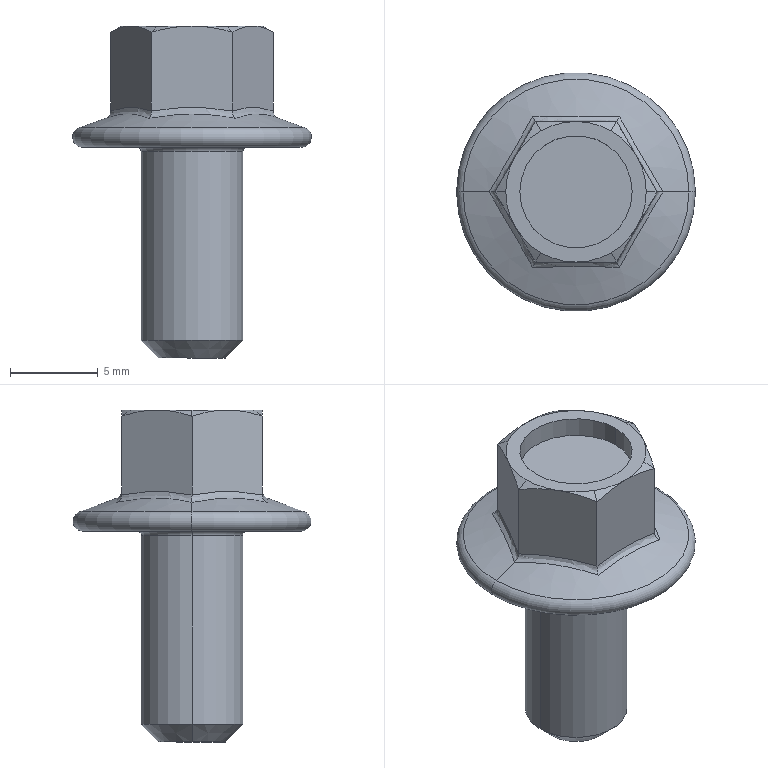Part | SolidWorks | features BaseBody 1 | 1 solid | 40 faces | box 13.6 x 13.6 x 18.9 mm | volume 775.835 mm3 | cone 16 | plane 10 | spline 6 | cylinder 4 | torus 4 | commonest cylinder face diameters 5.795 x2 6.4 x2